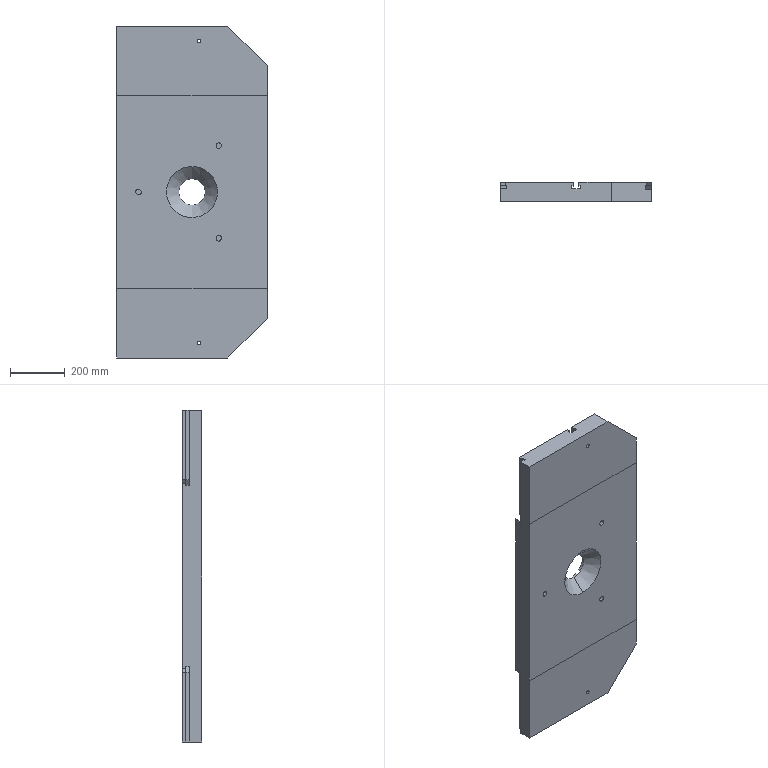Part | SolidWorks | features BaseBody 1 | 1 solid | 91 faces | box 550 x 70 x 1210 mm | volume 41984418 mm3 | plane 58 | cylinder 20 | spline 11 | cone 2 | commonest cylinder face diameters 20 x10 140 x6 13.5 x4